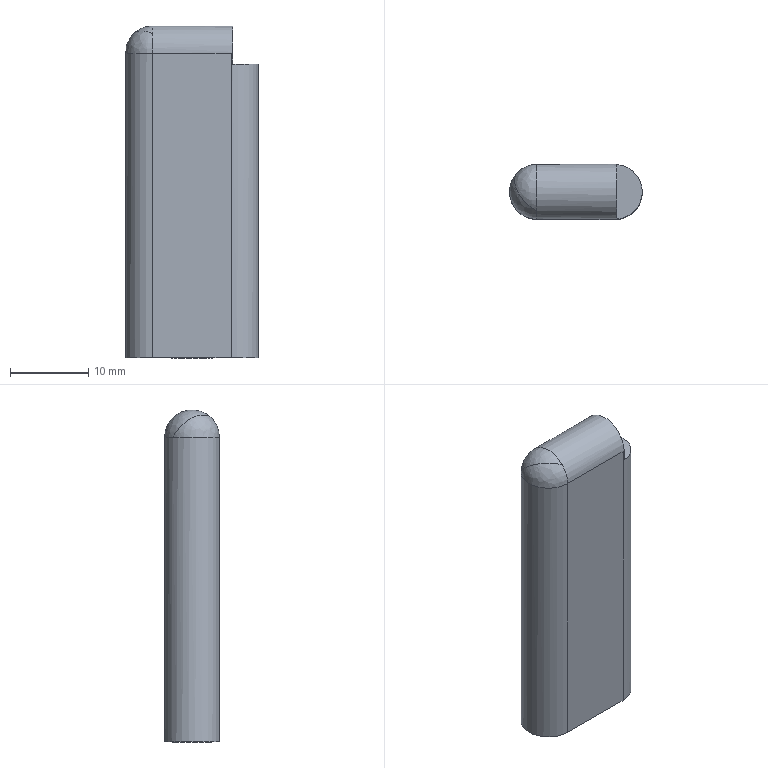Part | STEP file | LUOI GA TRON PHIA DUOI | 1 solid | 17 faces | box 17 x 7 x 42.5 mm | volume 4171 mm3 | cylinder 6 | plane 5 | cone 4 | spline 2 | commonest cylinder face diameters 7 x4 4.134 x2